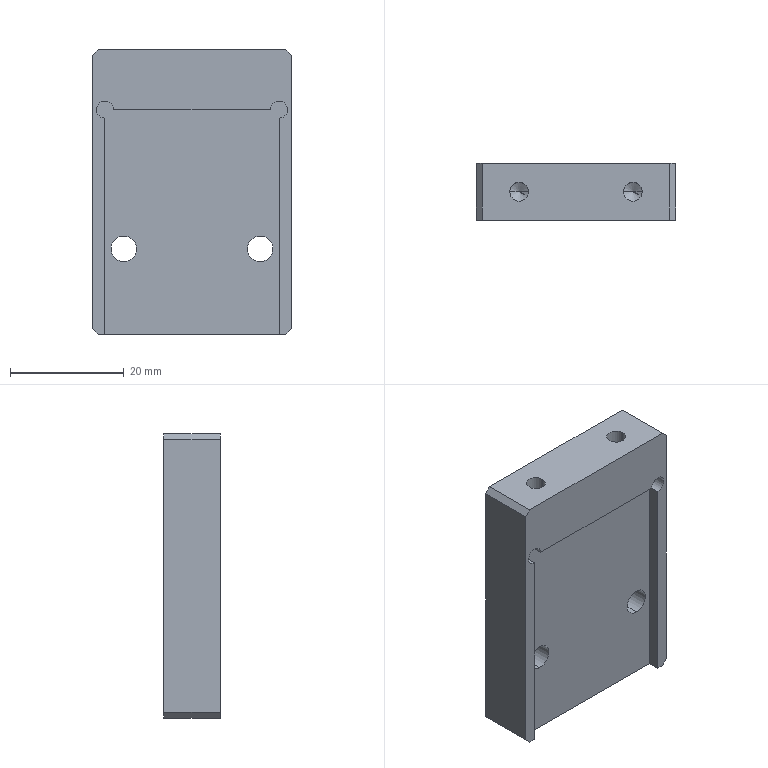Part | STEP file | PN_0014 | 1 solid | 34 faces | box 35 x 10 x 50 mm | volume 14292 mm3 | plane 16 | cylinder 14 | cone 4 | commonest cylinder face diameters 3.3 x4 4.5 x4 8 x4 3 x2